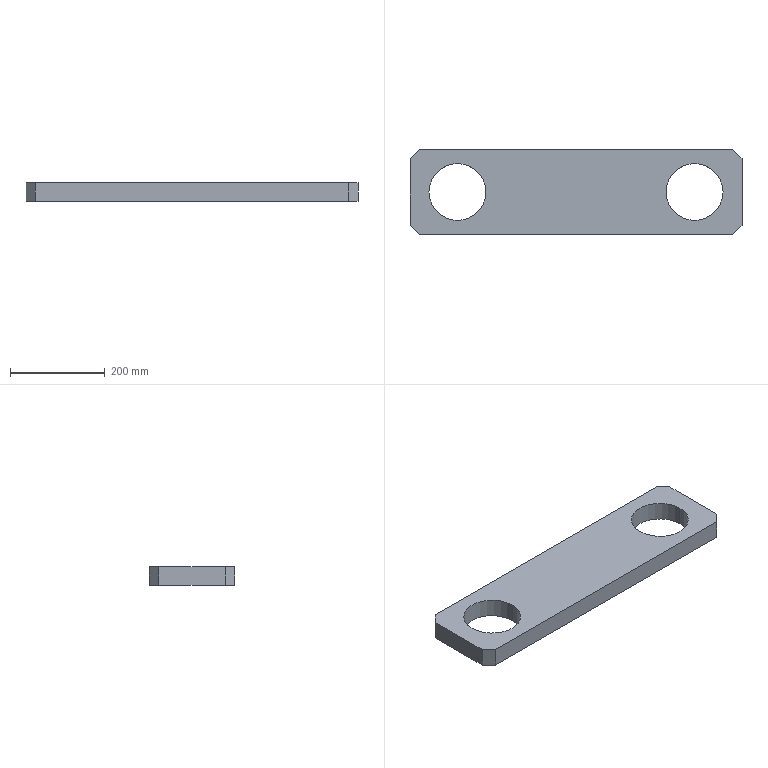Part | STEP file | 001-009-Riveting plate | 1 solid | 14 faces | box 700 x 180 x 40 mm | volume 4103221 mm3 | plane 10 | cylinder 4 | commonest cylinder face diameters 120 x4
STEP:
#1=CARTESIAN_POINT('',(0.,0.,0.));
#2=DIRECTION('',(0.,0.,1.));
#3=DIRECTION('',(1.,0.,0.));
#4=AXIS2_PLACEMENT_3D('',#1,#2,#3);
#5=CARTESIAN_POINT('',(-190.,0.,0.));
#6=VERTEX_POINT('',#5);
#7=CARTESIAN_POINT('',(-190.,0.,40.));
#8=VERTEX_POINT('',#7);
#9=CARTESIAN_POINT('',(-190.,0.,0.));
#10=DIRECTION('',(0.,0.,1.));
#11=VECTOR('',#10,1.);
#12=LINE('',#9,#11);
#13=CARTESIAN_POINT('',(-250.,0.,0.));
#14=DIRECTION('',(0.,0.,1.));
#15=DIRECTION('',(1.,0.,0.));
#16=AXIS2_PLACEMENT_3D('',#13,#14,#15);
#17=CYLINDRICAL_SURFACE('',#16,60.);
#18=CARTESIAN_POINT('',(6.283,0.));
#19=DIRECTION('',(0.,1.));
#20=VECTOR('',#19,1.);
#21=LINE('',#18,#20);
#22=(GEOMETRIC_REPRESENTATION_CONTEXT(2)PARAMETRIC_REPRESENTATION_CONTEXT()REPRESENTATION_CONTEXT('',''));
#23=DEFINITIONAL_REPRESENTATION('',(#21),#22);
#24=PCURVE('',#17,#23);
#25=CARTESIAN_POINT('',(-250.,0.,0.));
#26=DIRECTION('',(0.,0.,1.));
#27=DIRECTION('',(1.,0.,0.));
#28=AXIS2_PLACEMENT_3D('',#25,#26,#27);
#29=CYLINDRICAL_SURFACE('',#28,60.);
#30=CARTESIAN_POINT('',(0.,0.));
#31=DIRECTION('',(0.,1.));
#32=VECTOR('',#31,1.);
#33=LINE('',#30,#32);
#34=(GEOMETRIC_REPRESENTATION_CONTEXT(2)PARAMETRIC_REPRESENTATION_CONTEXT()REPRESENTATION_CONTEXT('',''));
#35=DEFINITIONAL_REPRESENTATION('',(#33),#34);
#36=PCURVE('',#29,#35);
#37=SURFACE_CURVE('',#12,(#24,#36),.PCURVE_S1.);
#38=EDGE_CURVE('',#6,#8,#37,.T.);
#39=ORIENTED_EDGE('',*,*,#38,.T.);
#40=CARTESIAN_POINT('',(-310.,0.,40.));
#41=VERTEX_POINT('',#40);
#42=CARTESIAN_POINT('',(-250.,0.,40.));
#43=DIRECTION('',(0.,0.,1.));
#44=DIRECTION('',(1.,0.,0.));
#45=AXIS2_PLACEMENT_3D('',#42,#43,#44);
#46=CIRCLE('',#45,60.);
#47=CARTESIAN_POINT('',(0.,40.));
#48=DIRECTION('',(1.,0.));
#49=VECTOR('',#48,1.);
#50=LINE('',#47,#49);
#51=(GEOMETRIC_REPRESENTATION_CONTEXT(2)PARAMETRIC_REPRESENTATION_CONTEXT()REPRESENTATION_CONTEXT('',''));
#52=DEFINITIONAL_REPRESENTATION('',(#50),#51);
#53=PCURVE('',#17,#52);
#54=CARTESIAN_POINT('',(0.,0.,40.));
#55=DIRECTION('',(0.,0.,1.));
#56=DIRECTION('',(1.,0.,0.));
#57=AXIS2_PLACEMENT_3D('',#54,#55,#56);
#58=PLANE('',#57);
#59=CARTESIAN_POINT('',(-250.,0.));
#60=DIRECTION('',(1.,0.));
#61=AXIS2_PLACEMENT_2D('',#59,#60);
#62=CIRCLE('',#61,60.);
#63=(GEOMETRIC_REPRESENTATION_CONTEXT(2)PARAMETRIC_REPRESENTATION_CONTEXT()REPRESENTATION_CONTEXT('',''));
#64=DEFINITIONAL_REPRESENTATION('',(#62),#63);
#65=PCURVE('',#58,#64);
#66=SURFACE_CURVE('',#46,(#53,#65),.PCURVE_S1.);
#67=EDGE_CURVE('',#41,#8,#66,.T.);
#68=ORIENTED_EDGE('',*,*,#67,.F.);
#69=CARTESIAN_POINT('',(-310.,0.,0.));
#70=VERTEX_POINT('',#69);
#71=CARTESIAN_POINT('',(-310.,0.,0.));
#72=DIRECTION('',(0.,0.,1.));
#73=VECTOR('',#72,1.);
#74=LINE('',#71,#73);
#75=CARTESIAN_POINT('',(3.142,0.));
#76=DIRECTION('',(0.,1.));
#77=VECTOR('',#76,1.);
#78=LINE('',#75,#77);
#79=(GEOMETRIC_REPRESENTATION_CONTEXT(2)PARAMETRIC_REPRESENTATION_CONTEXT()REPRESENTATION_CONTEXT('',''));
#80=DEFINITIONAL_REPRESENTATION('',(#78),#79);
#81=PCURVE('',#17,#80);
#82=CARTESIAN_POINT('',(3.142,0.));
#83=DIRECTION('',(0.,1.));
#84=VECTOR('',#83,1.);
#85=LINE('',#82,#84);
#86=(GEOMETRIC_REPRESENTATION_CONTEXT(2)PARAMETRIC_REPRESENTATION_CONTEXT()REPRESENTATION_CONTEXT('',''));
#87=DEFINITIONAL_REPRESENTATION('',(#85),#86);
#88=PCURVE('',#29,#87);
#89=SURFACE_CURVE('',#74,(#81,#88),.PCURVE_S1.);
#90=EDGE_CURVE('',#70,#41,#89,.T.);
#91=ORIENTED_EDGE('',*,*,#90,.F.);
#92=CARTESIAN_POINT('',(-250.,0.,0.));
#93=DIRECTION('',(0.,0.,1.));
#94=DIRECTION('',(1.,0.,0.));
#95=AXIS2_PLACEMENT_3D('',#92,#93,#94);
#96=CIRCLE('',#95,60.);
#97=CARTESIAN_POINT('',(0.,0.));
#98=DIRECTION('',(1.,0.));
#99=VECTOR('',#98,1.);
#100=LINE('',#97,#99);
#101=(GEOMETRIC_REPRESENTATION_CONTEXT(2)PARAMETRIC_REPRESENTATION_CONTEXT()REPRESENTATION_CONTEXT('',''));
#102=DEFINITIONAL_REPRESENTATION('',(#100),#101);
#103=PCURVE('',#17,#102);
#104=CARTESIAN_POINT('',(0.,0.,0.));
#105=DIRECTION('',(0.,0.,1.));
#106=DIRECTION('',(1.,0.,0.));
#107=AXIS2_PLACEMENT_3D('',#104,#105,#106);
#108=PLANE('',#107);
#109=CARTESIAN_POINT('',(-250.,0.));
#110=DIRECTION('',(1.,0.));
#111=AXIS2_PLACEMENT_2D('',#109,#110);
#112=CIRCLE('',#111,60.);
#113=(GEOMETRIC_REPRESENTATION_CONTEXT(2)PARAMETRIC_REPRESENTATION_CONTEXT()REPRESENTATION_CONTEXT('',''));
#114=DEFINITIONAL_REPRESENTATION('',(#112),#113);
#115=PCURVE('',#108,#114);
#116=SURFACE_CURVE('',#96,(#103,#115),.PCURVE_S1.);
#117=EDGE_CURVE('',#70,#6,#116,.T.);
#118=ORIENTED_EDGE('',*,*,#117,.T.);
#119=EDGE_LOOP('',(#39,#68,#91,#118));
#120=FACE_BOUND('',#119,.F.);
#121=ADVANCED_FACE('',(#120),#17,.F.);
#122=CARTESIAN_POINT('',(310.,0.,0.));
#123=VERTEX_POINT('',#122);
#124=CARTESIAN_POINT('',(310.,0.,40.));
#125=VERTEX_POINT('',#124);
#126=CARTESIAN_POINT('',(310.,0.,0.));
#127=DIRECTION('',(0.,0.,1.));
#128=VECTOR('',#127,1.);
#129=LINE('',#126,#128);
#130=CARTESIAN_POINT('',(250.,0.,0.));
#131=DIRECTION('',(0.,0.,1.));
#132=DIRECTION('',(1.,0.,0.));
#133=AXIS2_PLACEMENT_3D('',#130,#131,#132);
#134=CYLINDRICAL_SURFACE('',#133,60.);
#135=CARTESIAN_POINT('',(6.283,0.));
#136=DIRECTION('',(0.,1.));
#137=VECTOR('',#136,1.);
#138=LINE('',#135,#137);
#139=(GEOMETRIC_REPRESENTATION_CONTEXT(2)PARAMETRIC_REPRESENTATION_CONTEXT()REPRESENTATION_CONTEXT('',''));
#140=DEFINITIONAL_REPRESENTATION('',(#138),#139);
#141=PCURVE('',#134,#140);
#142=CARTESIAN_POINT('',(250.,0.,0.));
#143=DIRECTION('',(0.,0.,1.));
#144=DIRECTION('',(1.,0.,0.));
#145=AXIS2_PLACEMENT_3D('',#142,#143,#144);
#146=CYLINDRICAL_SURFACE('',#145,60.);
#147=CARTESIAN_POINT('',(0.,0.));
#148=DIRECTION('',(0.,1.));
#149=VECTOR('',#148,1.);
#150=LINE('',#147,#149);
#151=(GEOMETRIC_REPRESENTATION_CONTEXT(2)PARAMETRIC_REPRESENTATION_CONTEXT()REPRESENTATION_CONTEXT('',''));
#152=DEFINITIONAL_REPRESENTATION('',(#150),#151);
#153=PCURVE('',#146,#152);
#154=SURFACE_CURVE('',#129,(#141,#153),.PCURVE_S1.);
#155=EDGE_CURVE('',#123,#125,#154,.T.);
#156=ORIENTED_EDGE('',*,*,#155,.T.);
#157=CARTESIAN_POINT('',(190.,0.,40.));
#158=VERTEX_POINT('',#157);
#159=CARTESIAN_POINT('',(250.,0.,40.));
#160=DIRECTION('',(0.,0.,1.));
#161=DIRECTION('',(-1.,0.,0.));
#162=AXIS2_PLACEMENT_3D('',#159,#160,#161);
#163=CIRCLE('',#162,60.);
#164=CARTESIAN_POINT('',(3.142,40.));
#165=DIRECTION('',(1.,0.));
#166=VECTOR('',#165,1.);
#167=LINE('',#164,#166);
#168=(GEOMETRIC_REPRESENTATION_CONTEXT(2)PARAMETRIC_REPRESENTATION_CONTEXT()REPRESENTATION_CONTEXT('',''));
#169=DEFINITIONAL_REPRESENTATION('',(#167),#168);
#170=PCURVE('',#134,#169);
#171=CARTESIAN_POINT('',(250.,0.));
#172=DIRECTION('',(-1.,0.));
#173=AXIS2_PLACEMENT_2D('',#171,#172);
#174=CIRCLE('',#173,60.);
#175=(GEOMETRIC_REPRESENTATION_CONTEXT(2)PARAMETRIC_REPRESENTATION_CONTEXT()REPRESENTATION_CONTEXT('',''));
#176=DEFINITIONAL_REPRESENTATION('',(#174),#175);
#177=PCURVE('',#58,#176);
#178=SURFACE_CURVE('',#163,(#170,#177),.PCURVE_S1.);
#179=EDGE_CURVE('',#158,#125,#178,.T.);
#180=ORIENTED_EDGE('',*,*,#179,.F.);
#181=CARTESIAN_POINT('',(190.,0.,0.));
#182=VERTEX_POINT('',#181);
#183=CARTESIAN_POINT('',(190.,0.,0.));
#184=DIRECTION('',(0.,0.,1.));
#185=VECTOR('',#184,1.);
#186=LINE('',#183,#185);
#187=CARTESIAN_POINT('',(3.142,0.));
#188=DIRECTION('',(0.,1.));
#189=VECTOR('',#188,1.);
#190=LINE('',#187,#189);
#191=(GEOMETRIC_REPRESENTATION_CONTEXT(2)PARAMETRIC_REPRESENTATION_CONTEXT()REPRESENTATION_CONTEXT('',''));
#192=DEFINITIONAL_REPRESENTATION('',(#190),#191);
#193=PCURVE('',#134,#192);
#194=CARTESIAN_POINT('',(3.142,0.));
#195=DIRECTION('',(0.,1.));
#196=VECTOR('',#195,1.);
#197=LINE('',#194,#196);
#198=(GEOMETRIC_REPRESENTATION_CONTEXT(2)PARAMETRIC_REPRESENTATION_CONTEXT()REPRESENTATION_CONTEXT('',''));
#199=DEFINITIONAL_REPRESENTATION('',(#197),#198);
#200=PCURVE('',#146,#199);
#201=SURFACE_CURVE('',#186,(#193,#200),.PCURVE_S1.);
#202=EDGE_CURVE('',#182,#158,#201,.T.);
#203=ORIENTED_EDGE('',*,*,#202,.F.);
#204=CARTESIAN_POINT('',(250.,0.,0.));
#205=DIRECTION('',(0.,0.,1.));
#206=DIRECTION('',(-1.,0.,0.));
#207=AXIS2_PLACEMENT_3D('',#204,#205,#206);
#208=CIRCLE('',#207,60.);
#209=CARTESIAN_POINT('',(3.142,0.));
#210=DIRECTION('',(1.,0.));
#211=VECTOR('',#210,1.);
#212=LINE('',#209,#211);
#213=(GEOMETRIC_REPRESENTATION_CONTEXT(2)PARAMETRIC_REPRESENTATION_CONTEXT()REPRESENTATION_CONTEXT('',''));
#214=DEFINITIONAL_REPRESENTATION('',(#212),#213);
#215=PCURVE('',#134,#214);
#216=CARTESIAN_POINT('',(250.,0.));
#217=DIRECTION('',(-1.,0.));
#218=AXIS2_PLACEMENT_2D('',#216,#217);
#219=CIRCLE('',#218,60.);
#220=(GEOMETRIC_REPRESENTATION_CONTEXT(2)PARAMETRIC_REPRESENTATION_CONTEXT()REPRESENTATION_CONTEXT('',''));
#221=DEFINITIONAL_REPRESENTATION('',(#219),#220);
#222=PCURVE('',#108,#221);
#223=SURFACE_CURVE('',#208,(#215,#222),.PCURVE_S1.);
#224=EDGE_CURVE('',#182,#123,#223,.T.);
#225=ORIENTED_EDGE('',*,*,#224,.T.);
#226=EDGE_LOOP('',(#156,#180,#203,#225));
#227=FACE_BOUND('',#226,.F.);
#228=ADVANCED_FACE('',(#227),#134,.F.);
#229=CARTESIAN_POINT('',(350.,-70.,40.));
#230=VERTEX_POINT('',#229);
#231=CARTESIAN_POINT('',(350.,70.,40.));
#232=VERTEX_POINT('',#231);
#233=CARTESIAN_POINT('',(350.,90.,40.));
#234=DIRECTION('',(0.,1.,0.));
#235=VECTOR('',#234,1.);
#236=LINE('',#233,#235);
#237=CARTESIAN_POINT('',(350.,90.,40.));
#238=DIRECTION('',(-1.,0.,0.));
#239=DIRECTION('',(0.,0.,1.));
#240=AXIS2_PLACEMENT_3D('',#237,#238,#239);
#241=PLANE('',#240);
#242=CARTESIAN_POINT('',(0.,0.));
#243=DIRECTION('',(0.,1.));
#244=VECTOR('',#243,1.);
#245=LINE('',#242,#244);
#246=(GEOMETRIC_REPRESENTATION_CONTEXT(2)PARAMETRIC_REPRESENTATION_CONTEXT()REPRESENTATION_CONTEXT('',''));
#247=DEFINITIONAL_REPRESENTATION('',(#245),#246);
#248=PCURVE('',#241,#247);
#249=CARTESIAN_POINT('',(350.,90.));
#250=DIRECTION('',(0.,1.));
#251=VECTOR('',#250,1.);
#252=LINE('',#249,#251);
#253=(GEOMETRIC_REPRESENTATION_CONTEXT(2)PARAMETRIC_REPRESENTATION_CONTEXT()REPRESENTATION_CONTEXT('',''));
#254=DEFINITIONAL_REPRESENTATION('',(#252),#253);
#255=PCURVE('',#58,#254);
#256=SURFACE_CURVE('',#236,(#248,#255),.PCURVE_S1.);
#257=EDGE_CURVE('',#230,#232,#256,.T.);
#258=ORIENTED_EDGE('',*,*,#257,.F.);
#259=CARTESIAN_POINT('',(350.,-70.,0.));
#260=VERTEX_POINT('',#259);
#261=CARTESIAN_POINT('',(350.,-70.,40.));
#262=DIRECTION('',(0.,0.,-1.));
#263=VECTOR('',#262,1.);
#264=LINE('',#261,#263);
#265=CARTESIAN_POINT('',(0.,-160.));
#266=DIRECTION('',(-1.,0.));
#267=VECTOR('',#266,1.);
#268=LINE('',#265,#267);
#269=(GEOMETRIC_REPRESENTATION_CONTEXT(2)PARAMETRIC_REPRESENTATION_CONTEXT()REPRESENTATION_CONTEXT('',''));
#270=DEFINITIONAL_REPRESENTATION('',(#268),#269);
#271=PCURVE('',#241,#270);
#272=CARTESIAN_POINT('',(350.,-70.,40.));
#273=DIRECTION('',(-0.7071,0.7071,0.));
#274=DIRECTION('',(0.,0.,-1.));
#275=AXIS2_PLACEMENT_3D('',#272,#273,#274);
#276=PLANE('',#275);
#277=CARTESIAN_POINT('',(0.,0.));
#278=DIRECTION('',(1.,0.));
#279=VECTOR('',#278,1.);
#280=LINE('',#277,#279);
#281=(GEOMETRIC_REPRESENTATION_CONTEXT(2)PARAMETRIC_REPRESENTATION_CONTEXT()REPRESENTATION_CONTEXT('',''));
#282=DEFINITIONAL_REPRESENTATION('',(#280),#281);
#283=PCURVE('',#276,#282);
#284=SURFACE_CURVE('',#264,(#271,#283),.PCURVE_S1.);
#285=EDGE_CURVE('',#230,#260,#284,.T.);
#286=ORIENTED_EDGE('',*,*,#285,.T.);
#287=CARTESIAN_POINT('',(350.,70.,0.));
#288=VERTEX_POINT('',#287);
#289=CARTESIAN_POINT('',(350.,90.,0.));
#290=DIRECTION('',(0.,1.,0.));
#291=VECTOR('',#290,1.);
#292=LINE('',#289,#291);
#293=CARTESIAN_POINT('',(-40.,0.));
#294=DIRECTION('',(0.,1.));
#295=VECTOR('',#294,1.);
#296=LINE('',#293,#295);
#297=(GEOMETRIC_REPRESENTATION_CONTEXT(2)PARAMETRIC_REPRESENTATION_CONTEXT()REPRESENTATION_CONTEXT('',''));
#298=DEFINITIONAL_REPRESENTATION('',(#296),#297);
#299=PCURVE('',#241,#298);
#300=CARTESIAN_POINT('',(350.,90.));
#301=DIRECTION('',(0.,1.));
#302=VECTOR('',#301,1.);
#303=LINE('',#300,#302);
#304=(GEOMETRIC_REPRESENTATION_CONTEXT(2)PARAMETRIC_REPRESENTATION_CONTEXT()REPRESENTATION_CONTEXT('',''));
#305=DEFINITIONAL_REPRESENTATION('',(#303),#304);
#306=PCURVE('',#108,#305);
#307=SURFACE_CURVE('',#292,(#299,#306),.PCURVE_S1.);
#308=EDGE_CURVE('',#260,#288,#307,.T.);
#309=ORIENTED_EDGE('',*,*,#308,.T.);
#310=CARTESIAN_POINT('',(350.,70.,40.));
#311=DIRECTION('',(0.,0.,1.));
#312=VECTOR('',#311,1.);
#313=LINE('',#310,#312);
#314=CARTESIAN_POINT('',(0.,-20.));
#315=DIRECTION('',(1.,0.));
#316=VECTOR('',#315,1.);
#317=LINE('',#314,#316);
#318=(GEOMETRIC_REPRESENTATION_CONTEXT(2)PARAMETRIC_REPRESENTATION_CONTEXT()REPRESENTATION_CONTEXT('',''));
#319=DEFINITIONAL_REPRESENTATION('',(#317),#318);
#320=PCURVE('',#241,#319);
#321=CARTESIAN_POINT('',(330.,90.,40.));
#322=DIRECTION('',(-0.7071,-0.7071,0.));
#323=DIRECTION('',(0.,0.,-1.));
#324=AXIS2_PLACEMENT_3D('',#321,#322,#323);
#325=PLANE('',#324);
#326=CARTESIAN_POINT('',(0.,28.284));
#327=DIRECTION('',(-1.,0.));
#328=VECTOR('',#327,1.);
#329=LINE('',#326,#328);
#330=(GEOMETRIC_REPRESENTATION_CONTEXT(2)PARAMETRIC_REPRESENTATION_CONTEXT()REPRESENTATION_CONTEXT('',''));
#331=DEFINITIONAL_REPRESENTATION('',(#329),#330);
#332=PCURVE('',#325,#331);
#333=SURFACE_CURVE('',#313,(#320,#332),.PCURVE_S1.);
#334=EDGE_CURVE('',#288,#232,#333,.T.);
#335=ORIENTED_EDGE('',*,*,#334,.T.);
#336=EDGE_LOOP('',(#258,#286,#309,#335));
#337=FACE_BOUND('',#336,.T.);
#338=ADVANCED_FACE('',(#337),#241,.F.);
#339=CARTESIAN_POINT('',(330.,90.,40.));
#340=VERTEX_POINT('',#339);
#341=CARTESIAN_POINT('',(-330.,90.,40.));
#342=VERTEX_POINT('',#341);
#343=CARTESIAN_POINT('',(-350.,90.,40.));
#344=DIRECTION('',(-1.,0.,0.));
#345=VECTOR('',#344,1.);
#346=LINE('',#343,#345);
#347=CARTESIAN_POINT('',(-350.,90.,40.));
#348=DIRECTION('',(0.,-1.,0.));
#349=DIRECTION('',(1.,0.,0.));
#350=AXIS2_PLACEMENT_3D('',#347,#348,#349);
#351=PLANE('',#350);
#352=CARTESIAN_POINT('',(0.,0.));
#353=DIRECTION('',(-1.,0.));
#354=VECTOR('',#353,1.);
#355=LINE('',#352,#354);
#356=(GEOMETRIC_REPRESENTATION_CONTEXT(2)PARAMETRIC_REPRESENTATION_CONTEXT()REPRESENTATION_CONTEXT('',''));
#357=DEFINITIONAL_REPRESENTATION('',(#355),#356);
#358=PCURVE('',#351,#357);
#359=CARTESIAN_POINT('',(-350.,90.));
#360=DIRECTION('',(-1.,0.));
#361=VECTOR('',#360,1.);
#362=LINE('',#359,#361);
#363=(GEOMETRIC_REPRESENTATION_CONTEXT(2)PARAMETRIC_REPRESENTATION_CONTEXT()REPRESENTATION_CONTEXT('',''));
#364=DEFINITIONAL_REPRESENTATION('',(#362),#363);
#365=PCURVE('',#58,#364);
#366=SURFACE_CURVE('',#346,(#358,#365),.PCURVE_S1.);
#367=EDGE_CURVE('',#340,#342,#366,.T.);
#368=ORIENTED_EDGE('',*,*,#367,.F.);
#369=CARTESIAN_POINT('',(330.,90.,0.));
#370=VERTEX_POINT('',#369);
#371=CARTESIAN_POINT('',(330.,90.,40.));
#372=DIRECTION('',(0.,0.,-1.));
#373=VECTOR('',#372,1.);
#374=LINE('',#371,#373);
#375=CARTESIAN_POINT('',(680.,0.));
#376=DIRECTION('',(0.,-1.));
#377=VECTOR('',#376,1.);
#378=LINE('',#375,#377);
#379=(GEOMETRIC_REPRESENTATION_CONTEXT(2)PARAMETRIC_REPRESENTATION_CONTEXT()REPRESENTATION_CONTEXT('',''));
#380=DEFINITIONAL_REPRESENTATION('',(#378),#379);
#381=PCURVE('',#351,#380);
#382=CARTESIAN_POINT('',(0.,0.));
#383=DIRECTION('',(1.,0.));
#384=VECTOR('',#383,1.);
#385=LINE('',#382,#384);
#386=(GEOMETRIC_REPRESENTATION_CONTEXT(2)PARAMETRIC_REPRESENTATION_CONTEXT()REPRESENTATION_CONTEXT('',''));
#387=DEFINITIONAL_REPRESENTATION('',(#385),#386);
#388=PCURVE('',#325,#387);
#389=SURFACE_CURVE('',#374,(#381,#388),.PCURVE_S1.);
#390=EDGE_CURVE('',#340,#370,#389,.T.);
#391=ORIENTED_EDGE('',*,*,#390,.T.);
#392=CARTESIAN_POINT('',(-330.,90.,0.));
#393=VERTEX_POINT('',#392);
#394=CARTESIAN_POINT('',(-350.,90.,0.));
#395=DIRECTION('',(-1.,0.,0.));
#396=VECTOR('',#395,1.);
#397=LINE('',#394,#396);
#398=CARTESIAN_POINT('',(0.,-40.));
#399=DIRECTION('',(-1.,0.));
#400=VECTOR('',#399,1.);
#401=LINE('',#398,#400);
#402=(GEOMETRIC_REPRESENTATION_CONTEXT(2)PARAMETRIC_REPRESENTATION_CONTEXT()REPRESENTATION_CONTEXT('',''));
#403=DEFINITIONAL_REPRESENTATION('',(#401),#402);
#404=PCURVE('',#351,#403);
#405=CARTESIAN_POINT('',(-350.,90.));
#406=DIRECTION('',(-1.,0.));
#407=VECTOR('',#406,1.);
#408=LINE('',#405,#407);
#409=(GEOMETRIC_REPRESENTATION_CONTEXT(2)PARAMETRIC_REPRESENTATION_CONTEXT()REPRESENTATION_CONTEXT('',''));
#410=DEFINITIONAL_REPRESENTATION('',(#408),#409);
#411=PCURVE('',#108,#410);
#412=SURFACE_CURVE('',#397,(#404,#411),.PCURVE_S1.);
#413=EDGE_CURVE('',#370,#393,#412,.T.);
#414=ORIENTED_EDGE('',*,*,#413,.T.);
#415=CARTESIAN_POINT('',(-330.,90.,40.));
#416=DIRECTION('',(0.,0.,1.));
#417=VECTOR('',#416,1.);
#418=LINE('',#415,#417);
#419=CARTESIAN_POINT('',(20.,0.));
#420=DIRECTION('',(0.,1.));
#421=VECTOR('',#420,1.);
#422=LINE('',#419,#421);
#423=(GEOMETRIC_REPRESENTATION_CONTEXT(2)PARAMETRIC_REPRESENTATION_CONTEXT()REPRESENTATION_CONTEXT('',''));
#424=DEFINITIONAL_REPRESENTATION('',(#422),#423);
#425=PCURVE('',#351,#424);
#426=CARTESIAN_POINT('',(-350.,70.,40.));
#427=DIRECTION('',(0.7071,-0.7071,0.));
#428=DIRECTION('',(0.,0.,-1.));
#429=AXIS2_PLACEMENT_3D('',#426,#427,#428);
#430=PLANE('',#429);
#431=CARTESIAN_POINT('',(0.,28.284));
#432=DIRECTION('',(-1.,0.));
#433=VECTOR('',#432,1.);
#434=LINE('',#431,#433);
#435=(GEOMETRIC_REPRESENTATION_CONTEXT(2)PARAMETRIC_REPRESENTATION_CONTEXT()REPRESENTATION_CONTEXT('',''));
#436=DEFINITIONAL_REPRESENTATION('',(#434),#435);
#437=PCURVE('',#430,#436);
#438=SURFACE_CURVE('',#418,(#425,#437),.PCURVE_S1.);
#439=EDGE_CURVE('',#393,#342,#438,.T.);
#440=ORIENTED_EDGE('',*,*,#439,.T.);
#441=EDGE_LOOP('',(#368,#391,#414,#440));
#442=FACE_BOUND('',#441,.T.);
#443=ADVANCED_FACE('',(#442),#351,.F.);
#444=CARTESIAN_POINT('',(-350.,70.,0.));
#445=VERTEX_POINT('',#444);
#446=CARTESIAN_POINT('',(-350.,-70.,0.));
#447=VERTEX_POINT('',#446);
#448=CARTESIAN_POINT('',(-350.,90.,0.));
#449=DIRECTION('',(0.,-1.,0.));
#450=VECTOR('',#449,1.);
#451=LINE('',#448,#450);
#452=CARTESIAN_POINT('',(-350.,90.,40.));
#453=DIRECTION('',(1.,0.,0.));
#454=DIRECTION('',(0.,1.,0.));
#455=AXIS2_PLACEMENT_3D('',#452,#453,#454);
#456=PLANE('',#455);
#457=CARTESIAN_POINT('',(0.,-40.));
#458=DIRECTION('',(-1.,0.));
#459=VECTOR('',#458,1.);
#460=LINE('',#457,#459);
#461=(GEOMETRIC_REPRESENTATION_CONTEXT(2)PARAMETRIC_REPRESENTATION_CONTEXT()REPRESENTATION_CONTEXT('',''));
#462=DEFINITIONAL_REPRESENTATION('',(#460),#461);
#463=PCURVE('',#456,#462);
#464=CARTESIAN_POINT('',(-350.,90.));
#465=DIRECTION('',(0.,-1.));
#466=VECTOR('',#465,1.);
#467=LINE('',#464,#466);
#468=(GEOMETRIC_REPRESENTATION_CONTEXT(2)PARAMETRIC_REPRESENTATION_CONTEXT()REPRESENTATION_CONTEXT('',''));
#469=DEFINITIONAL_REPRESENTATION('',(#467),#468);
#470=PCURVE('',#108,#469);
#471=SURFACE_CURVE('',#451,(#463,#470),.PCURVE_S1.);
#472=EDGE_CURVE('',#445,#447,#471,.T.);
#473=ORIENTED_EDGE('',*,*,#472,.T.);
#474=CARTESIAN_POINT('',(-350.,-70.,40.));
#475=VERTEX_POINT('',#474);
#476=CARTESIAN_POINT('',(-350.,-70.,40.));
#477=DIRECTION('',(0.,0.,1.));
#478=VECTOR('',#477,1.);
#479=LINE('',#476,#478);
#480=CARTESIAN_POINT('',(-160.,0.));
#481=DIRECTION('',(0.,1.));
#482=VECTOR('',#481,1.);
#483=LINE('',#480,#482);
#484=(GEOMETRIC_REPRESENTATION_CONTEXT(2)PARAMETRIC_REPRESENTATION_CONTEXT()REPRESENTATION_CONTEXT('',''));
#485=DEFINITIONAL_REPRESENTATION('',(#483),#484);
#486=PCURVE('',#456,#485);
#487=CARTESIAN_POINT('',(-330.,-90.,40.));
#488=DIRECTION('',(0.7071,0.7071,0.));
#489=DIRECTION('',(0.,0.,-1.));
#490=AXIS2_PLACEMENT_3D('',#487,#488,#489);
#491=PLANE('',#490);
#492=CARTESIAN_POINT('',(0.,28.284));
#493=DIRECTION('',(-1.,0.));
#494=VECTOR('',#493,1.);
#495=LINE('',#492,#494);
#496=(GEOMETRIC_REPRESENTATION_CONTEXT(2)PARAMETRIC_REPRESENTATION_CONTEXT()REPRESENTATION_CONTEXT('',''));
#497=DEFINITIONAL_REPRESENTATION('',(#495),#496);
#498=PCURVE('',#491,#497);
#499=SURFACE_CURVE('',#479,(#486,#498),.PCURVE_S1.);
#500=EDGE_CURVE('',#447,#475,#499,.T.);
#501=ORIENTED_EDGE('',*,*,#500,.T.);
#502=CARTESIAN_POINT('',(-350.,70.,40.));
#503=VERTEX_POINT('',#502);
#504=CARTESIAN_POINT('',(-350.,90.,40.));
#505=DIRECTION('',(0.,-1.,0.));
#506=VECTOR('',#505,1.);
#507=LINE('',#504,#506);
#508=CARTESIAN_POINT('',(0.,0.));
#509=DIRECTION('',(-1.,0.));
#510=VECTOR('',#509,1.);
#511=LINE('',#508,#510);
#512=(GEOMETRIC_REPRESENTATION_CONTEXT(2)PARAMETRIC_REPRESENTATION_CONTEXT()REPRESENTATION_CONTEXT('',''));
#513=DEFINITIONAL_REPRESENTATION('',(#511),#512);
#514=PCURVE('',#456,#513);
#515=CARTESIAN_POINT('',(-350.,90.));
#516=DIRECTION('',(0.,-1.));
#517=VECTOR('',#516,1.);
#518=LINE('',#515,#517);
#519=(GEOMETRIC_REPRESENTATION_CONTEXT(2)PARAMETRIC_REPRESENTATION_CONTEXT()REPRESENTATION_CONTEXT('',''));
#520=DEFINITIONAL_REPRESENTATION('',(#518),#519);
#521=PCURVE('',#58,#520);
#522=SURFACE_CURVE('',#507,(#514,#521),.PCURVE_S1.);
#523=EDGE_CURVE('',#503,#475,#522,.T.);
#524=ORIENTED_EDGE('',*,*,#523,.F.);
#525=CARTESIAN_POINT('',(-350.,70.,40.));
#526=DIRECTION('',(0.,0.,-1.));
#527=VECTOR('',#526,1.);
#528=LINE('',#525,#527);
#529=CARTESIAN_POINT('',(-20.,0.));
#530=DIRECTION('',(0.,-1.));
#531=VECTOR('',#530,1.);
#532=LINE('',#529,#531);
#533=(GEOMETRIC_REPRESENTATION_CONTEXT(2)PARAMETRIC_REPRESENTATION_CONTEXT()REPRESENTATION_CONTEXT('',''));
#534=DEFINITIONAL_REPRESENTATION('',(#532),#533);
#535=PCURVE('',#456,#534);
#536=CARTESIAN_POINT('',(0.,0.));
#537=DIRECTION('',(1.,0.));
#538=VECTOR('',#537,1.);
#539=LINE('',#536,#538);
#540=(GEOMETRIC_REPRESENTATION_CONTEXT(2)PARAMETRIC_REPRESENTATION_CONTEXT()REPRESENTATION_CONTEXT('',''));
#541=DEFINITIONAL_REPRESENTATION('',(#539),#540);
#542=PCURVE('',#430,#541);
#543=SURFACE_CURVE('',#528,(#535,#542),.PCURVE_S1.);
#544=EDGE_CURVE('',#503,#445,#543,.T.);
#545=ORIENTED_EDGE('',*,*,#544,.T.);
#546=EDGE_LOOP('',(#473,#501,#524,#545));
#547=FACE_BOUND('',#546,.T.);
#548=ADVANCED_FACE('',(#547),#456,.F.);
#549=CARTESIAN_POINT('',(-330.,-90.,0.));
#550=VERTEX_POINT('',#549);
#551=CARTESIAN_POINT('',(330.,-90.,0.));
#552=VERTEX_POINT('',#551);
#553=CARTESIAN_POINT('',(-350.,-90.,0.));
#554=DIRECTION('',(1.,0.,0.));
#555=VECTOR('',#554,1.);
#556=LINE('',#553,#555);
#557=CARTESIAN_POINT('',(-350.,-90.,40.));
#558=DIRECTION('',(0.,1.,0.));
#559=DIRECTION('',(0.,0.,1.));
#560=AXIS2_PLACEMENT_3D('',#557,#558,#559);
#561=PLANE('',#560);
#562=CARTESIAN_POINT('',(-40.,0.));
#563=DIRECTION('',(0.,1.));
#564=VECTOR('',#563,1.);
#565=LINE('',#562,#564);
#566=(GEOMETRIC_REPRESENTATION_CONTEXT(2)PARAMETRIC_REPRESENTATION_CONTEXT()REPRESENTATION_CONTEXT('',''));
#567=DEFINITIONAL_REPRESENTATION('',(#565),#566);
#568=PCURVE('',#561,#567);
#569=CARTESIAN_POINT('',(-350.,-90.));
#570=DIRECTION('',(1.,0.));
#571=VECTOR('',#570,1.);
#572=LINE('',#569,#571);
#573=(GEOMETRIC_REPRESENTATION_CONTEXT(2)PARAMETRIC_REPRESENTATION_CONTEXT()REPRESENTATION_CONTEXT('',''));
#574=DEFINITIONAL_REPRESENTATION('',(#572),#573);
#575=PCURVE('',#108,#574);
#576=SURFACE_CURVE('',#556,(#568,#575),.PCURVE_S1.);
#577=EDGE_CURVE('',#550,#552,#576,.T.);
#578=ORIENTED_EDGE('',*,*,#577,.T.);
#579=CARTESIAN_POINT('',(330.,-90.,40.));
#580=VERTEX_POINT('',#579);
#581=CARTESIAN_POINT('',(330.,-90.,40.));
#582=DIRECTION('',(0.,0.,1.));
#583=VECTOR('',#582,1.);
#584=LINE('',#581,#583);
#585=CARTESIAN_POINT('',(0.,680.));
#586=DIRECTION('',(1.,0.));
#587=VECTOR('',#586,1.);
#588=LINE('',#585,#587);
#589=(GEOMETRIC_REPRESENTATION_CONTEXT(2)PARAMETRIC_REPRESENTATION_CONTEXT()REPRESENTATION_CONTEXT('',''));
#590=DEFINITIONAL_REPRESENTATION('',(#588),#589);
#591=PCURVE('',#561,#590);
#592=CARTESIAN_POINT('',(0.,28.284));
#593=DIRECTION('',(-1.,0.));
#594=VECTOR('',#593,1.);
#595=LINE('',#592,#594);
#596=(GEOMETRIC_REPRESENTATION_CONTEXT(2)PARAMETRIC_REPRESENTATION_CONTEXT()REPRESENTATION_CONTEXT('',''));
#597=DEFINITIONAL_REPRESENTATION('',(#595),#596);
#598=PCURVE('',#276,#597);
#599=SURFACE_CURVE('',#584,(#591,#598),.PCURVE_S1.);
#600=EDGE_CURVE('',#552,#580,#599,.T.);
#601=ORIENTED_EDGE('',*,*,#600,.T.);
#602=CARTESIAN_POINT('',(-330.,-90.,40.));
#603=VERTEX_POINT('',#602);
#604=CARTESIAN_POINT('',(-350.,-90.,40.));
#605=DIRECTION('',(1.,0.,0.));
#606=VECTOR('',#605,1.);
#607=LINE('',#604,#606);
#608=CARTESIAN_POINT('',(0.,0.));
#609=DIRECTION('',(0.,1.));
#610=VECTOR('',#609,1.);
#611=LINE('',#608,#610);
#612=(GEOMETRIC_REPRESENTATION_CONTEXT(2)PARAMETRIC_REPRESENTATION_CONTEXT()REPRESENTATION_CONTEXT('',''));
#613=DEFINITIONAL_REPRESENTATION('',(#611),#612);
#614=PCURVE('',#561,#613);
#615=CARTESIAN_POINT('',(-350.,-90.));
#616=DIRECTION('',(1.,0.));
#617=VECTOR('',#616,1.);
#618=LINE('',#615,#617);
#619=(GEOMETRIC_REPRESENTATION_CONTEXT(2)PARAMETRIC_REPRESENTATION_CONTEXT()REPRESENTATION_CONTEXT('',''));
#620=DEFINITIONAL_REPRESENTATION('',(#618),#619);
#621=PCURVE('',#58,#620);
#622=SURFACE_CURVE('',#607,(#614,#621),.PCURVE_S1.);
#623=EDGE_CURVE('',#603,#580,#622,.T.);
#624=ORIENTED_EDGE('',*,*,#623,.F.);
#625=CARTESIAN_POINT('',(-330.,-90.,40.));
#626=DIRECTION('',(0.,0.,-1.));
#627=VECTOR('',#626,1.);
#628=LINE('',#625,#627);
#629=CARTESIAN_POINT('',(0.,20.));
#630=DIRECTION('',(-1.,0.));
#631=VECTOR('',#630,1.);
#632=LINE('',#629,#631);
#633=(GEOMETRIC_REPRESENTATION_CONTEXT(2)PARAMETRIC_REPRESENTATION_CONTEXT()REPRESENTATION_CONTEXT('',''));
#634=DEFINITIONAL_REPRESENTATION('',(#632),#633);
#635=PCURVE('',#561,#634);
#636=CARTESIAN_POINT('',(0.,0.));
#637=DIRECTION('',(1.,0.));
#638=VECTOR('',#637,1.);
#639=LINE('',#636,#638);
#640=(GEOMETRIC_REPRESENTATION_CONTEXT(2)PARAMETRIC_REPRESENTATION_CONTEXT()REPRESENTATION_CONTEXT('',''));
#641=DEFINITIONAL_REPRESENTATION('',(#639),#640);
#642=PCURVE('',#491,#641);
#643=SURFACE_CURVE('',#628,(#635,#642),.PCURVE_S1.);
#644=EDGE_CURVE('',#603,#550,#643,.T.);
#645=ORIENTED_EDGE('',*,*,#644,.T.);
#646=EDGE_LOOP('',(#578,#601,#624,#645));
#647=FACE_BOUND('',#646,.T.);
#648=ADVANCED_FACE('',(#647),#561,.F.);
#649=CARTESIAN_POINT('',(-250.,0.,40.));
#650=DIRECTION('',(0.,0.,1.));
#651=DIRECTION('',(1.,0.,0.));
#652=AXIS2_PLACEMENT_3D('',#649,#650,#651);
#653=CIRCLE('',#652,60.);
#654=CARTESIAN_POINT('',(-250.,0.));
#655=DIRECTION('',(1.,0.));
#656=AXIS2_PLACEMENT_2D('',#654,#655);
#657=CIRCLE('',#656,60.);
#658=(GEOMETRIC_REPRESENTATION_CONTEXT(2)PARAMETRIC_REPRESENTATION_CONTEXT()REPRESENTATION_CONTEXT('',''));
#659=DEFINITIONAL_REPRESENTATION('',(#657),#658);
#660=PCURVE('',#58,#659);
#661=CARTESIAN_POINT('',(0.,40.));
#662=DIRECTION('',(1.,0.));
#663=VECTOR('',#662,1.);
#664=LINE('',#661,#663);
#665=(GEOMETRIC_REPRESENTATION_CONTEXT(2)PARAMETRIC_REPRESENTATION_CONTEXT()REPRESENTATION_CONTEXT('',''));
#666=DEFINITIONAL_REPRESENTATION('',(#664),#665);
#667=PCURVE('',#29,#666);
#668=SURFACE_CURVE('',#653,(#660,#667),.PCURVE_S1.);
#669=EDGE_CURVE('',#8,#41,#668,.T.);
#670=ORIENTED_EDGE('',*,*,#669,.F.);
#671=ORIENTED_EDGE('',*,*,#67,.F.);
#672=EDGE_LOOP('',(#670,#671));
#673=FACE_BOUND('',#672,.T.);
#674=CARTESIAN_POINT('',(250.,0.,40.));
#675=DIRECTION('',(0.,0.,1.));
#676=DIRECTION('',(-1.,0.,0.));
#677=AXIS2_PLACEMENT_3D('',#674,#675,#676);
#678=CIRCLE('',#677,60.);
#679=CARTESIAN_POINT('',(250.,0.));
#680=DIRECTION('',(-1.,0.));
#681=AXIS2_PLACEMENT_2D('',#679,#680);
#682=CIRCLE('',#681,60.);
#683=(GEOMETRIC_REPRESENTATION_CONTEXT(2)PARAMETRIC_REPRESENTATION_CONTEXT()REPRESENTATION_CONTEXT('',''));
#684=DEFINITIONAL_REPRESENTATION('',(#682),#683);
#685=PCURVE('',#58,#684);
#686=CARTESIAN_POINT('',(-3.142,40.));
#687=DIRECTION('',(1.,0.));
#688=VECTOR('',#687,1.);
#689=LINE('',#686,#688);
#690=(GEOMETRIC_REPRESENTATION_CONTEXT(2)PARAMETRIC_REPRESENTATION_CONTEXT()REPRESENTATION_CONTEXT('',''));
#691=DEFINITIONAL_REPRESENTATION('',(#689),#690);
#692=PCURVE('',#146,#691);
#693=SURFACE_CURVE('',#678,(#685,#692),.PCURVE_S1.);
#694=EDGE_CURVE('',#125,#158,#693,.T.);
#695=ORIENTED_EDGE('',*,*,#694,.F.);
#696=ORIENTED_EDGE('',*,*,#179,.F.);
#697=EDGE_LOOP('',(#695,#696));
#698=FACE_BOUND('',#697,.T.);
#699=ORIENTED_EDGE('',*,*,#623,.T.);
#700=CARTESIAN_POINT('',(210.,-210.,40.));
#701=DIRECTION('',(0.7071,0.7071,0.));
#702=VECTOR('',#701,1.);
#703=LINE('',#700,#702);
#704=CARTESIAN_POINT('',(210.,-210.));
#705=DIRECTION('',(0.7071,0.7071));
#706=VECTOR('',#705,1.);
#707=LINE('',#704,#706);
#708=(GEOMETRIC_REPRESENTATION_CONTEXT(2)PARAMETRIC_REPRESENTATION_CONTEXT()REPRESENTATION_CONTEXT('',''));
#709=DEFINITIONAL_REPRESENTATION('',(#707),#708);
#710=PCURVE('',#58,#709);
#711=CARTESIAN_POINT('',(0.,197.99));
#712=DIRECTION('',(0.,-1.));
#713=VECTOR('',#712,1.);
#714=LINE('',#711,#713);
#715=(GEOMETRIC_REPRESENTATION_CONTEXT(2)PARAMETRIC_REPRESENTATION_CONTEXT()REPRESENTATION_CONTEXT('',''));
#716=DEFINITIONAL_REPRESENTATION('',(#714),#715);
#717=PCURVE('',#276,#716);
#718=SURFACE_CURVE('',#703,(#710,#717),.PCURVE_S1.);
#719=EDGE_CURVE('',#580,#230,#718,.T.);
#720=ORIENTED_EDGE('',*,*,#719,.T.);
#721=ORIENTED_EDGE('',*,*,#257,.T.);
#722=CARTESIAN_POINT('',(210.,210.,40.));
#723=DIRECTION('',(-0.7071,0.7071,0.));
#724=VECTOR('',#723,1.);
#725=LINE('',#722,#724);
#726=CARTESIAN_POINT('',(210.,210.));
#727=DIRECTION('',(-0.7071,0.7071));
#728=VECTOR('',#727,1.);
#729=LINE('',#726,#728);
#730=(GEOMETRIC_REPRESENTATION_CONTEXT(2)PARAMETRIC_REPRESENTATION_CONTEXT()REPRESENTATION_CONTEXT('',''));
#731=DEFINITIONAL_REPRESENTATION('',(#729),#730);
#732=PCURVE('',#58,#731);
#733=CARTESIAN_POINT('',(0.,-169.706));
#734=DIRECTION('',(0.,-1.));
#735=VECTOR('',#734,1.);
#736=LINE('',#733,#735);
#737=(GEOMETRIC_REPRESENTATION_CONTEXT(2)PARAMETRIC_REPRESENTATION_CONTEXT()REPRESENTATION_CONTEXT('',''));
#738=DEFINITIONAL_REPRESENTATION('',(#736),#737);
#739=PCURVE('',#325,#738);
#740=SURFACE_CURVE('',#725,(#732,#739),.PCURVE_S1.);
#741=EDGE_CURVE('',#232,#340,#740,.T.);
#742=ORIENTED_EDGE('',*,*,#741,.T.);
#743=ORIENTED_EDGE('',*,*,#367,.T.);
#744=CARTESIAN_POINT('',(-210.,210.,40.));
#745=DIRECTION('',(-0.7071,-0.7071,0.));
#746=VECTOR('',#745,1.);
#747=LINE('',#744,#746);
#748=CARTESIAN_POINT('',(-210.,210.));
#749=DIRECTION('',(-0.7071,-0.7071));
#750=VECTOR('',#749,1.);
#751=LINE('',#748,#750);
#752=(GEOMETRIC_REPRESENTATION_CONTEXT(2)PARAMETRIC_REPRESENTATION_CONTEXT()REPRESENTATION_CONTEXT('',''));
#753=DEFINITIONAL_REPRESENTATION('',(#751),#752);
#754=PCURVE('',#58,#753);
#755=CARTESIAN_POINT('',(0.,197.99));
#756=DIRECTION('',(0.,-1.));
#757=VECTOR('',#756,1.);
#758=LINE('',#755,#757);
#759=(GEOMETRIC_REPRESENTATION_CONTEXT(2)PARAMETRIC_REPRESENTATION_CONTEXT()REPRESENTATION_CONTEXT('',''));
#760=DEFINITIONAL_REPRESENTATION('',(#758),#759);
#761=PCURVE('',#430,#760);
#762=SURFACE_CURVE('',#747,(#754,#761),.PCURVE_S1.);
#763=EDGE_CURVE('',#342,#503,#762,.T.);
#764=ORIENTED_EDGE('',*,*,#763,.T.);
#765=ORIENTED_EDGE('',*,*,#523,.T.);
#766=CARTESIAN_POINT('',(-210.,-210.,40.));
#767=DIRECTION('',(0.7071,-0.7071,0.));
#768=VECTOR('',#767,1.);
#769=LINE('',#766,#768);
#770=CARTESIAN_POINT('',(-210.,-210.));
#771=DIRECTION('',(0.7071,-0.7071));
#772=VECTOR('',#771,1.);
#773=LINE('',#770,#772);
#774=(GEOMETRIC_REPRESENTATION_CONTEXT(2)PARAMETRIC_REPRESENTATION_CONTEXT()REPRESENTATION_CONTEXT('',''));
#775=DEFINITIONAL_REPRESENTATION('',(#773),#774);
#776=PCURVE('',#58,#775);
#777=CARTESIAN_POINT('',(0.,-169.706));
#778=DIRECTION('',(0.,-1.));
#779=VECTOR('',#778,1.);
#780=LINE('',#777,#779);
#781=(GEOMETRIC_REPRESENTATION_CONTEXT(2)PARAMETRIC_REPRESENTATION_CONTEXT()REPRESENTATION_CONTEXT('',''));
#782=DEFINITIONAL_REPRESENTATION('',(#780),#781);
#783=PCURVE('',#491,#782);
#784=SURFACE_CURVE('',#769,(#776,#783),.PCURVE_S1.);
#785=EDGE_CURVE('',#475,#603,#784,.T.);
#786=ORIENTED_EDGE('',*,*,#785,.T.);
#787=EDGE_LOOP('',(#699,#720,#721,#742,#743,#764,#765,#786));
#788=FACE_BOUND('',#787,.T.);
#789=ADVANCED_FACE('',(#673,#698,#788),#58,.T.);
#790=CARTESIAN_POINT('',(-250.,0.,0.));
#791=DIRECTION('',(0.,0.,1.));
#792=DIRECTION('',(1.,0.,0.));
#793=AXIS2_PLACEMENT_3D('',#790,#791,#792);
#794=CIRCLE('',#793,60.);
#795=CARTESIAN_POINT('',(-250.,0.));
#796=DIRECTION('',(1.,0.));
#797=AXIS2_PLACEMENT_2D('',#795,#796);
#798=CIRCLE('',#797,60.);
#799=(GEOMETRIC_REPRESENTATION_CONTEXT(2)PARAMETRIC_REPRESENTATION_CONTEXT()REPRESENTATION_CONTEXT('',''));
#800=DEFINITIONAL_REPRESENTATION('',(#798),#799);
#801=PCURVE('',#108,#800);
#802=CARTESIAN_POINT('',(0.,0.));
#803=DIRECTION('',(1.,0.));
#804=VECTOR('',#803,1.);
#805=LINE('',#802,#804);
#806=(GEOMETRIC_REPRESENTATION_CONTEXT(2)PARAMETRIC_REPRESENTATION_CONTEXT()REPRESENTATION_CONTEXT('',''));
#807=DEFINITIONAL_REPRESENTATION('',(#805),#806);
#808=PCURVE('',#29,#807);
#809=SURFACE_CURVE('',#794,(#801,#808),.PCURVE_S1.);
#810=EDGE_CURVE('',#6,#70,#809,.T.);
#811=ORIENTED_EDGE('',*,*,#810,.T.);
#812=ORIENTED_EDGE('',*,*,#117,.T.);
#813=EDGE_LOOP('',(#811,#812));
#814=FACE_BOUND('',#813,.T.);
#815=CARTESIAN_POINT('',(250.,0.,0.));
#816=DIRECTION('',(0.,0.,1.));
#817=DIRECTION('',(-1.,0.,0.));
#818=AXIS2_PLACEMENT_3D('',#815,#816,#817);
#819=CIRCLE('',#818,60.);
#820=CARTESIAN_POINT('',(250.,0.));
#821=DIRECTION('',(-1.,0.));
#822=AXIS2_PLACEMENT_2D('',#820,#821);
#823=CIRCLE('',#822,60.);
#824=(GEOMETRIC_REPRESENTATION_CONTEXT(2)PARAMETRIC_REPRESENTATION_CONTEXT()REPRESENTATION_CONTEXT('',''));
#825=DEFINITIONAL_REPRESENTATION('',(#823),#824);
#826=PCURVE('',#108,#825);
#827=CARTESIAN_POINT('',(-3.142,0.));
#828=DIRECTION('',(1.,0.));
#829=VECTOR('',#828,1.);
#830=LINE('',#827,#829);
#831=(GEOMETRIC_REPRESENTATION_CONTEXT(2)PARAMETRIC_REPRESENTATION_CONTEXT()REPRESENTATION_CONTEXT('',''));
#832=DEFINITIONAL_REPRESENTATION('',(#830),#831);
#833=PCURVE('',#146,#832);
#834=SURFACE_CURVE('',#819,(#826,#833),.PCURVE_S1.);
#835=EDGE_CURVE('',#123,#182,#834,.T.);
#836=ORIENTED_EDGE('',*,*,#835,.T.);
#837=ORIENTED_EDGE('',*,*,#224,.T.);
#838=EDGE_LOOP('',(#836,#837));
#839=FACE_BOUND('',#838,.T.);
#840=ORIENTED_EDGE('',*,*,#308,.F.);
#841=CARTESIAN_POINT('',(350.,-70.,0.));
#842=DIRECTION('',(-0.7071,-0.7071,0.));
#843=VECTOR('',#842,1.);
#844=LINE('',#841,#843);
#845=CARTESIAN_POINT('',(350.,-70.));
#846=DIRECTION('',(-0.7071,-0.7071));
#847=VECTOR('',#846,1.);
#848=LINE('',#845,#847);
#849=(GEOMETRIC_REPRESENTATION_CONTEXT(2)PARAMETRIC_REPRESENTATION_CONTEXT()REPRESENTATION_CONTEXT('',''));
#850=DEFINITIONAL_REPRESENTATION('',(#848),#849);
#851=PCURVE('',#108,#850);
#852=CARTESIAN_POINT('',(40.,0.));
#853=DIRECTION('',(0.,1.));
#854=VECTOR('',#853,1.);
#855=LINE('',#852,#854);
#856=(GEOMETRIC_REPRESENTATION_CONTEXT(2)PARAMETRIC_REPRESENTATION_CONTEXT()REPRESENTATION_CONTEXT('',''));
#857=DEFINITIONAL_REPRESENTATION('',(#855),#856);
#858=PCURVE('',#276,#857);
#859=SURFACE_CURVE('',#844,(#851,#858),.PCURVE_S1.);
#860=EDGE_CURVE('',#260,#552,#859,.T.);
#861=ORIENTED_EDGE('',*,*,#860,.T.);
#862=ORIENTED_EDGE('',*,*,#577,.F.);
#863=CARTESIAN_POINT('',(-330.,-90.,0.));
#864=DIRECTION('',(-0.7071,0.7071,0.));
#865=VECTOR('',#864,1.);
#866=LINE('',#863,#865);
#867=CARTESIAN_POINT('',(-330.,-90.));
#868=DIRECTION('',(-0.7071,0.7071));
#869=VECTOR('',#868,1.);
#870=LINE('',#867,#869);
#871=(GEOMETRIC_REPRESENTATION_CONTEXT(2)PARAMETRIC_REPRESENTATION_CONTEXT()REPRESENTATION_CONTEXT('',''));
#872=DEFINITIONAL_REPRESENTATION('',(#870),#871);
#873=PCURVE('',#108,#872);
#874=CARTESIAN_POINT('',(40.,0.));
#875=DIRECTION('',(0.,1.));
#876=VECTOR('',#875,1.);
#877=LINE('',#874,#876);
#878=(GEOMETRIC_REPRESENTATION_CONTEXT(2)PARAMETRIC_REPRESENTATION_CONTEXT()REPRESENTATION_CONTEXT('',''));
#879=DEFINITIONAL_REPRESENTATION('',(#877),#878);
#880=PCURVE('',#491,#879);
#881=SURFACE_CURVE('',#866,(#873,#880),.PCURVE_S1.);
#882=EDGE_CURVE('',#550,#447,#881,.T.);
#883=ORIENTED_EDGE('',*,*,#882,.T.);
#884=ORIENTED_EDGE('',*,*,#472,.F.);
#885=CARTESIAN_POINT('',(-350.,70.,0.));
#886=DIRECTION('',(0.7071,0.7071,0.));
#887=VECTOR('',#886,1.);
#888=LINE('',#885,#887);
#889=CARTESIAN_POINT('',(-350.,70.));
#890=DIRECTION('',(0.7071,0.7071));
#891=VECTOR('',#890,1.);
#892=LINE('',#889,#891);
#893=(GEOMETRIC_REPRESENTATION_CONTEXT(2)PARAMETRIC_REPRESENTATION_CONTEXT()REPRESENTATION_CONTEXT('',''));
#894=DEFINITIONAL_REPRESENTATION('',(#892),#893);
#895=PCURVE('',#108,#894);
#896=CARTESIAN_POINT('',(40.,0.));
#897=DIRECTION('',(0.,1.));
#898=VECTOR('',#897,1.);
#899=LINE('',#896,#898);
#900=(GEOMETRIC_REPRESENTATION_CONTEXT(2)PARAMETRIC_REPRESENTATION_CONTEXT()REPRESENTATION_CONTEXT('',''));
#901=DEFINITIONAL_REPRESENTATION('',(#899),#900);
#902=PCURVE('',#430,#901);
#903=SURFACE_CURVE('',#888,(#895,#902),.PCURVE_S1.);
#904=EDGE_CURVE('',#445,#393,#903,.T.);
#905=ORIENTED_EDGE('',*,*,#904,.T.);
#906=ORIENTED_EDGE('',*,*,#413,.F.);
#907=CARTESIAN_POINT('',(330.,90.,0.));
#908=DIRECTION('',(0.7071,-0.7071,0.));
#909=VECTOR('',#908,1.);
#910=LINE('',#907,#909);
#911=CARTESIAN_POINT('',(330.,90.));
#912=DIRECTION('',(0.7071,-0.7071));
#913=VECTOR('',#912,1.);
#914=LINE('',#911,#913);
#915=(GEOMETRIC_REPRESENTATION_CONTEXT(2)PARAMETRIC_REPRESENTATION_CONTEXT()REPRESENTATION_CONTEXT('',''));
#916=DEFINITIONAL_REPRESENTATION('',(#914),#915);
#917=PCURVE('',#108,#916);
#918=CARTESIAN_POINT('',(40.,0.));
#919=DIRECTION('',(0.,1.));
#920=VECTOR('',#919,1.);
#921=LINE('',#918,#920);
#922=(GEOMETRIC_REPRESENTATION_CONTEXT(2)PARAMETRIC_REPRESENTATION_CONTEXT()REPRESENTATION_CONTEXT('',''));
#923=DEFINITIONAL_REPRESENTATION('',(#921),#922);
#924=PCURVE('',#325,#923);
#925=SURFACE_CURVE('',#910,(#917,#924),.PCURVE_S1.);
#926=EDGE_CURVE('',#370,#288,#925,.T.);
#927=ORIENTED_EDGE('',*,*,#926,.T.);
#928=EDGE_LOOP('',(#840,#861,#862,#883,#884,#905,#906,#927));
#929=FACE_BOUND('',#928,.T.);
#930=ADVANCED_FACE('',(#814,#839,#929),#108,.F.);
#931=ORIENTED_EDGE('',*,*,#719,.F.);
#932=ORIENTED_EDGE('',*,*,#600,.F.);
#933=ORIENTED_EDGE('',*,*,#860,.F.);
#934=ORIENTED_EDGE('',*,*,#285,.F.);
#935=EDGE_LOOP('',(#931,#932,#933,#934));
#936=FACE_BOUND('',#935,.T.);
#937=ADVANCED_FACE('',(#936),#276,.F.);
#938=ORIENTED_EDGE('',*,*,#785,.F.);
#939=ORIENTED_EDGE('',*,*,#500,.F.);
#940=ORIENTED_EDGE('',*,*,#882,.F.);
#941=ORIENTED_EDGE('',*,*,#644,.F.);
#942=EDGE_LOOP('',(#938,#939,#940,#941));
#943=FACE_BOUND('',#942,.T.);
#944=ADVANCED_FACE('',(#943),#491,.F.);
#945=ORIENTED_EDGE('',*,*,#741,.F.);
#946=ORIENTED_EDGE('',*,*,#334,.F.);
#947=ORIENTED_EDGE('',*,*,#926,.F.);
#948=ORIENTED_EDGE('',*,*,#390,.F.);
#949=EDGE_LOOP('',(#945,#946,#947,#948));
#950=FACE_BOUND('',#949,.T.);
#951=ADVANCED_FACE('',(#950),#325,.F.);
#952=ORIENTED_EDGE('',*,*,#763,.F.);
#953=ORIENTED_EDGE('',*,*,#439,.F.);
#954=ORIENTED_EDGE('',*,*,#904,.F.);
#955=ORIENTED_EDGE('',*,*,#544,.F.);
#956=EDGE_LOOP('',(#952,#953,#954,#955));
#957=FACE_BOUND('',#956,.T.);
#958=ADVANCED_FACE('',(#957),#430,.F.);
#959=ORIENTED_EDGE('',*,*,#694,.F.);
#960=ORIENTED_EDGE('',*,*,#155,.F.);
#961=ORIENTED_EDGE('',*,*,#835,.T.);
#962=ORIENTED_EDGE('',*,*,#202,.T.);
#963=EDGE_LOOP('',(#959,#960,#961,#962));
#964=FACE_BOUND('',#963,.F.);
#965=ADVANCED_FACE('',(#964),#146,.F.);
#966=ORIENTED_EDGE('',*,*,#669,.F.);
#967=ORIENTED_EDGE('',*,*,#38,.F.);
#968=ORIENTED_EDGE('',*,*,#810,.T.);
#969=ORIENTED_EDGE('',*,*,#90,.T.);
#970=EDGE_LOOP('',(#966,#967,#968,#969));
#971=FACE_BOUND('',#970,.F.);
#972=ADVANCED_FACE('',(#971),#29,.F.);
#973=CLOSED_SHELL('',(#121,#228,#338,#443,#548,#648,#789,#930,#937,#944,#951,#958,#965,#972));
#974=MANIFOLD_SOLID_BREP('',#973);
#975=(LENGTH_UNIT()NAMED_UNIT(*)SI_UNIT(.MILLI.,.METRE.));
#976=UNCERTAINTY_MEASURE_WITH_UNIT(LENGTH_MEASURE(0.0000001),#975,'','');
#977=(NAMED_UNIT(*)PLANE_ANGLE_UNIT()SI_UNIT($,.RADIAN.));
#978=(NAMED_UNIT(*)SI_UNIT($,.STERADIAN.)SOLID_ANGLE_UNIT());
#979=(GEOMETRIC_REPRESENTATION_CONTEXT(3)GLOBAL_UNCERTAINTY_ASSIGNED_CONTEXT((#976))GLOBAL_UNIT_ASSIGNED_CONTEXT((#975,#977,#978))REPRESENTATION_CONTEXT('',''));
#980=ADVANCED_BREP_SHAPE_REPRESENTATION('',(#4,#974),#979);